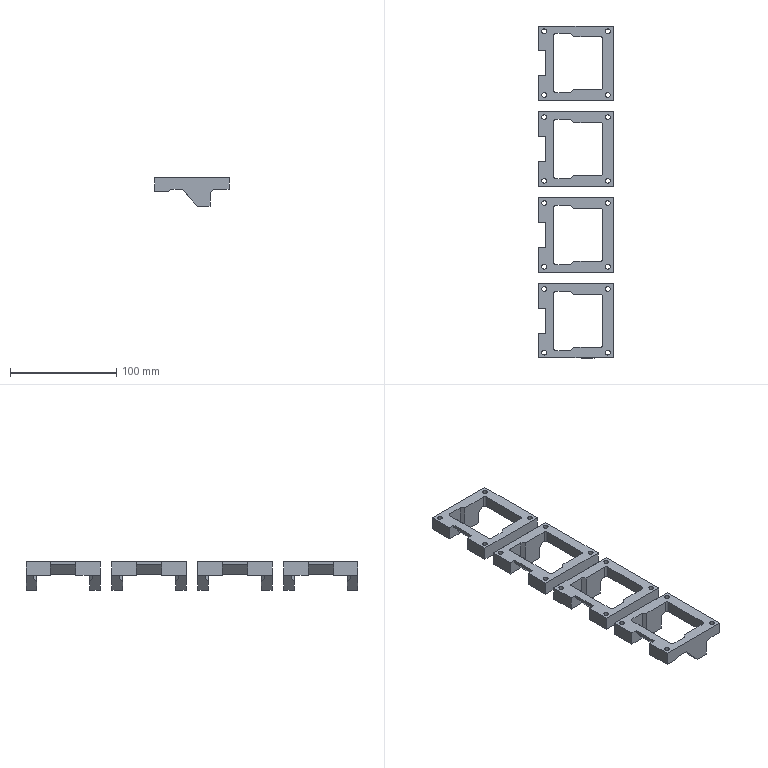NC program | NX | posted with a generic post | part box 70 x 313 x 26.9 mm
Lines 23251 to 24227 of 34421:
(CAVITY_MILL_COPY , TOOL : D4)
N46476 T04 M6
N46478 G54
N46480 G17 G0 G90 X145.982 Y5.441 S9500 M3
N46482 G43 Z30. H4
N46484 Z-11.1
N46486 G94 G1 Z-11.6 F1000.
N46488 X146.316 Y5.352
N46490 G3 X147.282 Y5.611 R1.
N46492 G1 X147.69 Y6.018 F1500.
N46494 G2 X147.987 Y6.482 R1.989
N46496 G3 X148.172 Y7.464 R1.
N46498 G1 X148.12 Y7.612
N46500 Z-11.1
N46502 G0 X145.602 Y5.062 Z-11.5
N46504 G1 Z-12. F1000.
N46506 X145.937 Y4.972
N46508 G3 X146.903 Y5.231 R1.
N46510 G1 X147.529 Y5.857 F1500.
N46512 G2 X147.789 Y6.558 R2.001
N46514 G3 X147.81 Y7.558 R1.
N46516 G1 X147.734 Y7.695
N46518 Z-11.5
N46520 G0 X145.414 Y4.874 Z-11.9
N46522 G1 Z-12.4 F1000.
N46524 X145.749 Y4.784
N46526 G3 X146.714 Y5.043 R1.
N46528 G1 X147.506 Y5.835 F1500.
N46530 G2 X147.681 Y6.704 R1.968
N46532 G3 X147.583 Y7.699 R1.
N46534 G1 X147.493 Y7.825
N46536 Z-11.9
N46538 G0 X145.304 Y4.764 Z-12.3
N46540 G1 Z-12.8 F1000.
N46542 X145.638 Y4.674
N46544 G3 X146.604 Y4.933 R1.
N46546 G1 X147.506 Y5.835 F1500.
N46548 X147.5 Y5.88
N46550 Y6.218
N46552 G2 X147.606 Y6.861 R2.
N46554 G3 X147.411 Y7.842 R1.
N46556 G1 X147.308 Y7.96
N46558 Z-12.3
N46560 G0 X145.243 Y4.703 Z-12.7
N46562 G1 Z-13.2 F1000.
N46564 X145.578 Y4.614
N46566 G3 X146.544 Y4.872 R1.
N46568 G1 X147.506 Y5.835 F1500.
N46570 X147.5 Y5.88
N46572 Y6.566
N46574 G2 X147.559 Y7.046 R2.
N46576 G3 X147.281 Y8.007 R1.
N46578 G1 X147.168 Y8.116
N46580 Z-12.7
N46582 G0 X145.219 Y4.679 Z-13.1
N46584 G1 Z-13.6 F1000.
N46586 X145.553 Y4.589
N46588 G3 X146.519 Y4.848 R1.
N46590 G1 X147.503 Y5.831 F1500.
N46592 X147.5 Y5.88
N46594 Y6.914
N46596 G2 X147.518 Y7.18 R2.
N46598 G3 X147.137 Y8.105 R1.
N46600 G1 X147.013 Y8.2
N46602 Z-13.1
N46604 G0 X145.215 Y4.675 Z-13.5
N46606 G1 Z-14. F1000.
N46608 X145.55 Y4.585
N46610 G3 X146.516 Y4.844 R1.
N46612 G1 X147.503 Y5.831 F1500.
N46614 X147.5 Y5.88
N46616 Y7.206
N46618 G3 X147. Y8.072 R1.
N46620 G1 X146.849 Y8.159
N46622 Z-13.5
N46624 G0 X145.215 Y4.675 Z-13.9
N46626 G1 Z-14.4 F1000.
N46628 X145.55 Y4.585
N46630 G3 X146.516 Y4.844 R1.
N46632 G1 X147.502 Y5.831 F1500.
N46634 X147.5 Y5.88
N46636 Y7.206
N46638 G3 X147. Y8.072 R1.
N46640 G1 X146.765 Y8.208
N46642 Z-13.9
N46644 G0 X145.215 Y4.675 Z-14.3
N46646 G1 Z-14.8 F1000.
N46648 X145.55 Y4.585
N46650 G3 X146.516 Y4.844 R1.
N46652 G1 X147.502 Y5.831 F1500.
N46654 X147.5 Y5.88
N46656 Y7.206
N46658 G3 X147. Y8.072 R1.
N46660 G1 X146.714 Y8.238
N46662 Z-14.3
N46664 G0 X145.215 Y4.675 Z-14.7
N46666 G1 Z-15.2 F1000.
N46668 X145.55 Y4.585
N46670 G3 X146.515 Y4.844 R1.
N46672 G1 X147.502 Y5.831 F1500.
N46674 X147.5 Y5.88
N46676 Y7.207
N46678 G3 X147. Y8.073 R1.
N46680 G1 X146.7 Y8.246
N46682 Z-14.7
N46684 G0 X145.215 Y4.675 Z-15.1
N46686 G1 Z-15.6 F1000.
N46688 X145.549 Y4.585
N46690 G3 X146.515 Y4.844 R1.
N46692 G1 X147.502 Y5.831 F1500.
N46694 X147.5 Y5.88
N46696 Y7.207
N46698 G3 X147. Y8.073 R1.
N46700 G1 X146.7 Y8.247
N46702 Z-15.1
N46704 G0 X145.215 Y4.675 Z-15.5
N46706 G1 Z-16. F1000.
N46708 X145.549 Y4.585
N46710 G3 X146.515 Y4.844 R1.
N46712 G1 X147.502 Y5.831 F1500.
N46714 X147.5 Y5.88
N46716 Y7.208
N46718 G3 X147. Y8.074 R1.
N46720 G1 X146.7 Y8.247
N46722 Z-15.5
N46724 G0 X145.215 Y4.675 Z-15.889
N46726 G1 Z-16.389 F1000.
N46728 X145.549 Y4.585
N46730 G3 X146.515 Y4.844 R1.
N46732 G1 X147.502 Y5.831 F1500.
N46734 X147.5 Y5.88
N46736 Y7.208
N46738 G3 X147. Y8.074 R1.
N46740 G1 X146.7 Y8.247
N46742 Z-15.889
N46744 G0 X145.215 Y4.674 Z-16.279
N46746 G1 Z-16.779 F1000.
N46748 X145.549 Y4.585
N46750 G3 X146.515 Y4.844 R1.
N46752 G1 X147.502 Y5.831 F1500.
N46754 X147.5 Y5.88
N46756 Y7.209
N46758 G3 X147. Y8.075 R1.
N46760 G1 X146.7 Y8.248
N46762 Z-16.279
N46764 G0 X145.215 Y4.674 Z-16.668
N46766 G1 Z-17.168 F1000.
N46768 X145.549 Y4.585
N46770 G3 X146.515 Y4.844 R1.
N46772 G1 X147.502 Y5.831 F1500.
N46774 X147.5 Y5.88
N46776 Y7.209
N46778 G3 X147. Y8.075 R1.
N46780 G1 X146.7 Y8.248
N46782 Z-16.668
N46784 G0 X145.215 Y4.674 Z-17.057
N46786 G1 Z-17.557 F1000.
N46788 X145.549 Y4.585
N46790 G3 X146.515 Y4.843 R1.
N46792 G1 X147.502 Y5.83 F1500.
N46794 X147.5 Y5.88
N46796 Y7.21
N46798 G3 X147. Y8.076 R1.
N46800 G1 X146.7 Y8.249
N46802 Z-17.057
N46804 G0 X145.214 Y4.674 Z-17.446
N46806 G1 Z-17.946 F1000.
N46808 X145.549 Y4.585
N46810 G3 X146.515 Y4.843 R1.
N46812 G1 X147.502 Y5.83 F1500.
N46814 X147.5 Y5.88
N46816 Y7.21
N46818 G3 X147. Y8.076 R1.
N46820 G1 X146.7 Y8.249
N46822 Z-17.446
N46824 G0 X145.214 Y4.674 Z-17.836
N46826 G1 Z-18.336 F1000.
N46828 X145.549 Y4.585
N46830 G3 X146.515 Y4.843 R1.
N46832 G1 X147.502 Y5.83 F1500.
N46834 X147.5 Y5.88
N46836 Y7.21
N46838 G3 X147. Y8.076 R1.
N46840 G1 X146.7 Y8.25
N46842 Z-17.836
N46844 G0 X145.214 Y4.674 Z-18.225
N46846 G1 Z-18.725 F1000.
N46848 X145.549 Y4.584
N46850 G3 X146.515 Y4.843 R1.
N46852 G1 X147.502 Y5.83 F1500.
N46854 X147.5 Y5.88
N46856 Y7.211
N46858 G3 X147. Y8.077 R1.
N46860 G1 X146.7 Y8.25
N46862 Z-18.225
N46864 G0 X145.214 Y4.674 Z-18.614
N46866 G1 Z-19.114 F1000.
N46868 X145.549 Y4.584
N46870 G3 X146.515 Y4.843 R1.
N46872 G1 X147.502 Y5.83 F1500.
N46874 X147.5 Y5.88
N46876 Y7.211
N46878 G3 X147. Y8.077 R1.
N46880 G1 X146.7 Y8.251
N46882 Z-18.614
N46884 G0 X145.214 Y4.674 Z-19.004
N46886 G1 Z-19.504 F1000.
N46888 X145.549 Y4.584
N46890 G3 X146.515 Y4.843 R1.
N46892 G1 X147.502 Y5.83 F1500.
N46894 X147.5 Y5.88
N46896 Y7.212
N46898 G3 X147. Y8.078 R1.
N46900 G1 X146.7 Y8.251
N46902 Z-19.004
N46904 G0 X145.214 Y4.674 Z-19.393
N46906 G1 Z-19.893 F1000.
N46908 X145.549 Y4.584
N46910 G3 X146.515 Y4.843 R1.
N46912 G1 X147.502 Y5.83 F1500.
N46914 X147.5 Y5.88
N46916 Y7.212
N46918 G3 X147. Y8.078 R1.
N46920 G1 X146.7 Y8.251
N46922 Z-19.393
N46924 G0 X145.214 Y4.674 Z-19.782
N46926 G1 Z-20.282 F1000.
N46928 X145.549 Y4.584
N46930 G3 X146.515 Y4.843 R1.
N46932 G1 X147.502 Y5.83 F1500.
N46934 X147.5 Y5.88
N46936 Y7.213
N46938 G3 X147. Y8.079 R1.
N46940 G1 X146.7 Y8.252
N46942 Z-19.782
N46944 G0 X145.214 Y4.674 Z-20.171
N46946 G1 Z-20.671 F1000.
N46948 X145.549 Y4.584
N46950 G3 X146.515 Y4.843 R1.
N46952 G1 X147.502 Y5.83 F1500.
N46954 X147.5 Y5.88
N46956 Y7.213
N46958 G3 X147. Y8.079 R1.
N46960 G1 X146.7 Y8.252
N46962 Z-20.171
N46964 G0 X145.214 Y4.674 Z-20.561
N46966 G1 Z-21.061 F1000.
N46968 X145.549 Y4.584
N46970 G3 X146.515 Y4.843 R1.
N46972 G1 X147.502 Y5.83 F1500.
N46974 X147.5 Y5.88
N46976 Y7.214
N46978 G3 X147. Y8.08 R1.
N46980 G1 X146.7 Y8.253
N46982 Z-20.561
N46984 G0 X145.214 Y4.674 Z-20.95
N46986 G1 Z-21.45 F1000.
N46988 X145.549 Y4.584
N46990 G3 X146.514 Y4.843 R1.
N46992 G1 X147.501 Y5.83 F1500.
N46994 X147.5 Y5.88
N46996 Y7.214
N46998 G3 X147. Y8.08 R1.
N47000 G1 X146.7 Y8.253
N47002 Z-20.95
N47004 G0 X145.214 Y4.674 Z-21.339
N47006 G1 Z-21.839 F1000.
N47008 X145.548 Y4.584
N47010 G3 X146.514 Y4.843 R1.
N47012 G1 X147.501 Y5.83 F1500.
N47014 X147.5 Y5.88
N47016 Y7.214
N47018 G3 X147. Y8.081 R1.
N47020 G1 X146.7 Y8.254
N47022 Z-21.339
N47024 G0 X145.214 Y4.674 Z-21.729
N47026 G1 Z-22.229 F1000.
N47028 X145.548 Y4.584
N47030 G3 X146.514 Y4.843 R1.
N47032 G1 X147.501 Y5.83 F1500.
N47034 X147.5 Y5.88
N47036 Y7.215
N47038 G3 X147. Y8.081 R1.
N47040 G1 X146.7 Y8.254
N47042 Z-21.729
N47044 G0 X145.214 Y4.674 Z-22.118
N47046 G1 Z-22.618 F1000.
N47048 X145.548 Y4.584
N47050 G3 X146.514 Y4.843 R1.
N47052 G1 X147.501 Y5.83 F1500.
N47054 X147.5 Y5.88
N47056 Y7.215
N47058 G3 X147. Y8.081 R1.
N47060 G1 X146.7 Y8.255
N47062 Z-22.118
N47064 G0 X145.214 Y4.673 Z-22.507
N47066 G1 Z-23.007 F1000.
N47068 X145.548 Y4.584
N47070 G3 X146.514 Y4.843 R1.
N47072 G1 X147.501 Y5.83 F1500.
N47074 X147.5 Y5.88
N47076 Y7.216
N47078 G3 X147. Y8.082 R1.
N47080 G1 X146.7 Y8.255
N47082 Z-22.507
N47084 G0 X145.214 Y4.673 Z-22.896
N47086 G1 Z-23.396 F1000.
N47088 X145.548 Y4.584
N47090 G3 X146.514 Y4.843 R1.
N47092 G1 X147.501 Y5.83 F1500.
N47094 X147.5 Y5.88
N47096 Y7.216
N47098 G3 X147. Y8.082 R1.
N47100 G1 X146.7 Y8.256
N47102 Z-22.896
N47104 G0 X145.214 Y4.673 Z-23.286
N47106 G1 Z-23.786 F1000.
N47108 X145.548 Y4.584
N47110 G3 X146.514 Y4.843 R1.
N47112 G1 X147.501 Y5.83 F1500.
N47114 X147.5 Y5.88
N47116 Y7.217
N47118 G3 X147. Y8.083 R1.
N47120 G1 X146.7 Y8.256
N47122 Z-23.286
N47124 G0 X145.214 Y4.673 Z-23.675
N47126 G1 Z-24.175 F1000.
N47128 X145.548 Y4.584
N47130 G3 X146.514 Y4.842 R1.
N47132 G1 X147.501 Y5.83 F1500.
N47134 X147.5 Y5.88
N47136 Y7.217
N47138 G3 X147. Y8.083 R1.
N47140 G1 X146.7 Y8.256
N47142 Z-23.675
N47144 G0 X145.213 Y4.673 Z-24.064
N47146 G1 Z-24.564 F1000.
N47148 X145.548 Y4.584
N47150 G3 X146.514 Y4.842 R1.
N47152 G1 X147.501 Y5.829 F1500.
N47154 X147.5 Y5.88
N47156 Y7.218
N47158 G3 X147. Y8.084 R1.
N47160 G1 X146.7 Y8.257
N47162 Z-24.064
N47164 G0 X145.213 Y4.673 Z-24.454
N47166 G1 Z-24.954 F1000.
N47168 X145.548 Y4.584
N47170 G3 X146.514 Y4.842 R1.
N47172 G1 X147.501 Y5.829 F1500.
N47174 X147.5 Y5.88
N47176 Y7.218
N47178 G3 X147. Y8.084 R1.
N47180 G1 X146.7 Y8.257
N47182 Z-24.454
N47184 G0 X145.213 Y4.673 Z-24.843
N47186 G1 Z-25.343 F1000.
N47188 X145.548 Y4.583
N47190 G3 X146.514 Y4.842 R1.
N47192 G1 X147.501 Y5.829 F1500.
N47194 X147.5 Y5.88
N47196 Y7.219
N47198 G3 X147. Y8.085 R1.
N47200 G1 X146.7 Y8.258
N47202 Z-24.843
N47204 G0 X145.213 Y4.673 Z-25.232
N47206 G1 Z-25.732 F1000.
N47208 X145.548 Y4.583
N47210 G3 X146.514 Y4.842 R1.
N47212 G1 X147.501 Y5.829 F1500.
N47214 X147.5 Y5.88
N47216 Y7.219
N47218 G3 X147. Y8.085 R1.
N47220 G1 X146.7 Y8.258
N47222 Z-25.232
N47224 G0 X145.213 Y4.673 Z-25.621
N47226 G1 Z-26.121 F1000.
N47228 X145.548 Y4.583
N47230 G3 X146.514 Y4.842 R1.
N47232 G1 X147.501 Y5.829 F1500.
N47234 X147.5 Y5.88
N47236 Y7.219
N47238 G3 X147. Y8.085 R1.
N47240 G1 X146.7 Y8.259
N47242 Z-25.621
N47244 G0 X145.213 Y4.673 Z-26.011
N47246 G1 Z-26.511 F1000.
N47248 X145.548 Y4.583
N47250 G3 X146.514 Y4.842 R1.
N47252 G1 X147.501 Y5.829 F1500.
N47254 X147.5 Y5.88
N47256 Y7.22
N47258 G3 X147. Y8.086 R1.
N47260 G1 X146.7 Y8.259
N47262 Z-26.011
N47264 G0 X145.213 Y4.673 Z-26.4
N47266 G1 Z-26.9 F1000.
N47268 X145.548 Y4.583
N47270 G3 X146.514 Y4.842 R1.
N47272 G1 X147.501 Y5.829 F1500.
N47274 X147.5 Y5.88
N47276 Y7.22
N47278 G3 X147. Y8.086 R1.
N47280 G1 X146.7 Y8.26
N47282 Z-26.4
N47284 G0 Z30.
N47286 X148.906 Y17.66
N47288 Z-15.1
N47290 G1 Z-15.6 F1000.
N47292 X148.875 Y17.817
N47294 G3 X148.217 Y18.571 R1.
N47296 G2 X147.493 Y19. R2.058 F1500.
N47298 G1 X146.455
N47300 G3 X145.589 Y18.5 R1.
N47302 G1 X145.415 Y18.2
N47304 Z-15.1
N47306 G0 X148.788 Y17.239 Z-15.5
N47308 G1 Z-16. F1000.
N47310 X148.784 Y17.398
N47312 G3 X148.265 Y18.253 R1.
N47314 G2 X147.493 Y19. R2.029 F1500.
N47316 G1 X146.081
N47318 G3 X145.215 Y18.5 R1.
N47320 G1 X145.041 Y18.2
N47322 Z-15.5
N47324 G0 X146.7 Y14.808 Z-15.889
N47326 G1 Z-16.389 F1000.
N47328 X147. Y14.981
N47330 G3 X147.5 Y15.847 R1.
N47332 G1 Y18.988 F1500.
N47334 X147.493 Y19.
N47336 X144.347
N47338 G3 X143.481 Y18.5 R1.
N47340 G1 X143.308 Y18.2
N47342 Z-15.889
N47344 G0 X146.7 Y14.808 Z-16.279
N47346 G1 Z-16.779 F1000.
N47348 X147. Y14.981
N47350 G3 X147.5 Y15.847 R1.
N47352 G1 Y18.988 F1500.
N47354 X147.493 Y19.
N47356 X144.347
N47358 G3 X143.481 Y18.5 R1.
N47360 G1 X143.308 Y18.2
N47362 Z-16.279
N47364 G0 X146.7 Y14.808 Z-16.668
N47366 G1 Z-17.168 F1000.
N47368 X147. Y14.981
N47370 G3 X147.5 Y15.847 R1.
N47372 G1 Y18.988 F1500.
N47374 X147.493 Y19.
N47376 X144.347
N47378 G3 X143.481 Y18.5 R1.
N47380 G1 X143.308 Y18.2
N47382 Z-16.668
N47384 G0 X146.7 Y14.808 Z-17.057
N47386 G1 Z-17.557 F1000.
N47388 X147. Y14.981
N47390 G3 X147.5 Y15.847 R1.
N47392 G1 Y18.988 F1500.
N47394 X147.493 Y19.
N47396 X144.347
N47398 G3 X143.481 Y18.5 R1.
N47400 G1 X143.308 Y18.2
N47402 Z-17.057
N47404 G0 X146.7 Y14.808 Z-17.446
N47406 G1 Z-17.946 F1000.
N47408 X147. Y14.981
N47410 G3 X147.5 Y15.847 R1.
N47412 G1 Y18.988 F1500.
N47414 X147.493 Y19.
N47416 X144.347
N47418 G3 X143.481 Y18.5 R1.
N47420 G1 X143.308 Y18.2
N47422 Z-17.446
N47424 G0 X146.7 Y14.808 Z-17.836
N47426 G1 Z-18.336 F1000.
N47428 X147. Y14.981
N47430 G3 X147.5 Y15.847 R1.
N47432 G1 Y18.988 F1500.
N47434 X147.493 Y19.
N47436 X144.347
N47438 G3 X143.481 Y18.5 R1.
N47440 G1 X143.308 Y18.2
N47442 Z-17.836
N47444 G0 X146.7 Y14.808 Z-18.225
N47446 G1 Z-18.725 F1000.
N47448 X147. Y14.981
N47450 G3 X147.5 Y15.847 R1.
N47452 G1 Y18.988 F1500.
N47454 X147.492 Y19.
N47456 X144.347
N47458 G3 X143.481 Y18.5 R1.
N47460 G1 X143.308 Y18.2
N47462 Z-18.225
N47464 G0 X146.7 Y14.808 Z-18.614
N47466 G1 Z-19.114 F1000.
N47468 X147. Y14.981
N47470 G3 X147.5 Y15.847 R1.
N47472 G1 Y18.988 F1500.
N47474 X147.492 Y19.
N47476 X144.347
N47478 G3 X143.481 Y18.5 R1.
N47480 G1 X143.308 Y18.2
N47482 Z-18.614
N47484 G0 X146.7 Y14.808 Z-19.004
N47486 G1 Z-19.504 F1000.
N47488 X147. Y14.981
N47490 G3 X147.5 Y15.847 R1.
N47492 G1 Y18.988 F1500.
N47494 X147.492 Y19.
N47496 X144.347
N47498 G3 X143.481 Y18.5 R1.
N47500 G1 X143.308 Y18.2
N47502 Z-19.004
N47504 G0 X146.7 Y14.808 Z-19.393
N47506 G1 Z-19.893 F1000.
N47508 X147. Y14.981
N47510 G3 X147.5 Y15.847 R1.
N47512 G1 Y18.988 F1500.
N47514 X147.492 Y19.
N47516 X144.347
N47518 G3 X143.481 Y18.5 R1.
N47520 G1 X143.308 Y18.2
N47522 Z-19.393
N47524 G0 X146.7 Y14.808 Z-19.782
N47526 G1 Z-20.282 F1000.
N47528 X147. Y14.981
N47530 G3 X147.5 Y15.847 R1.
N47532 G1 Y18.988 F1500.
N47534 X147.492 Y19.
N47536 X144.347
N47538 G3 X143.481 Y18.5 R1.
N47540 G1 X143.308 Y18.2
N47542 Z-19.782
N47544 G0 X146.7 Y14.808 Z-20.171
N47546 G1 Z-20.671 F1000.
N47548 X147. Y14.981
N47550 G3 X147.5 Y15.847 R1.
N47552 G1 Y18.988 F1500.
N47554 X147.492 Y19.
N47556 X144.347
N47558 G3 X143.481 Y18.5 R1.
N47560 G1 X143.308 Y18.2
N47562 Z-20.171
N47564 G0 X146.7 Y14.808 Z-20.561
N47566 G1 Z-21.061 F1000.
N47568 X147. Y14.981
N47570 G3 X147.5 Y15.847 R1.
N47572 G1 Y18.988 F1500.
N47574 X147.492 Y19.
N47576 X144.347
N47578 G3 X143.481 Y18.5 R1.
N47580 G1 X143.308 Y18.2
N47582 Z-20.561
N47584 G0 X146.7 Y14.808 Z-20.95
N47586 G1 Z-21.45 F1000.
N47588 X147. Y14.981
N47590 G3 X147.5 Y15.847 R1.
N47592 G1 Y18.988 F1500.
N47594 X147.492 Y19.
N47596 X144.347
N47598 G3 X143.481 Y18.5 R1.
N47600 G1 X143.308 Y18.2
N47602 Z-20.95
N47604 G0 X146.7 Y14.808 Z-21.339
N47606 G1 Z-21.839 F1000.
N47608 X147. Y14.981
N47610 G3 X147.5 Y15.847 R1.
N47612 G1 Y18.988 F1500.
N47614 X147.492 Y19.
N47616 X144.347
N47618 G3 X143.481 Y18.5 R1.
N47620 G1 X143.308 Y18.2
N47622 Z-21.339
N47624 G0 X146.7 Y14.808 Z-21.729
N47626 G1 Z-22.229 F1000.
N47628 X147. Y14.981
N47630 G3 X147.5 Y15.847 R1.
N47632 G1 Y18.988 F1500.
N47634 X147.492 Y19.
N47636 X144.347
N47638 G3 X143.481 Y18.5 R1.
N47640 G1 X143.308 Y18.2
N47642 Z-21.729
N47644 G0 X146.7 Y14.808 Z-22.118
N47646 G1 Z-22.618 F1000.
N47648 X147. Y14.981
N47650 G3 X147.5 Y15.847 R1.
N47652 G1 Y18.988 F1500.
N47654 X147.492 Y19.
N47656 X144.347
N47658 G3 X143.481 Y18.5 R1.
N47660 G1 X143.308 Y18.2
N47662 Z-22.118
N47664 G0 X146.7 Y14.808 Z-22.507
N47666 G1 Z-23.007 F1000.
N47668 X147. Y14.981
N47670 G3 X147.5 Y15.847 R1.
N47672 G1 Y18.988 F1500.
N47674 X147.492 Y19.
N47676 X144.347
N47678 G3 X143.481 Y18.5 R1.
N47680 G1 X143.308 Y18.2
N47682 Z-22.507
N47684 G0 X146.7 Y14.808 Z-22.896
N47686 G1 Z-23.396 F1000.
N47688 X147. Y14.981
N47690 G3 X147.5 Y15.847 R1.
N47692 G1 Y18.988 F1500.
N47694 X147.492 Y19.
N47696 X144.347
N47698 G3 X143.481 Y18.5 R1.
N47700 G1 X143.308 Y18.2
N47702 Z-22.896
N47704 G0 X146.7 Y14.808 Z-23.286
N47706 G1 Z-23.786 F1000.
N47708 X147. Y14.981
N47710 G3 X147.5 Y15.847 R1.
N47712 G1 Y18.988 F1500.
N47714 X147.492 Y19.
N47716 X144.347
N47718 G3 X143.481 Y18.5 R1.
N47720 G1 X143.308 Y18.2
N47722 Z-23.286
N47724 G0 X146.7 Y14.808 Z-23.675
N47726 G1 Z-24.175 F1000.
N47728 X147. Y14.981
N47730 G3 X147.5 Y15.847 R1.
N47732 G1 Y18.988 F1500.
N47734 X147.491 Y19.
N47736 X144.347
N47738 G3 X143.481 Y18.5 R1.
N47740 G1 X143.308 Y18.2
N47742 Z-23.675
N47744 G0 X146.7 Y14.808 Z-24.064
N47746 G1 Z-24.564 F1000.
N47748 X147. Y14.981
N47750 G3 X147.5 Y15.847 R1.
N47752 G1 Y18.988 F1500.
N47754 X147.491 Y19.
N47756 X144.347
N47758 G3 X143.481 Y18.5 R1.
N47760 G1 X143.308 Y18.2
N47762 Z-24.064
N47764 G0 X146.7 Y14.808 Z-24.454
N47766 G1 Z-24.954 F1000.
N47768 X147. Y14.981
N47770 G3 X147.5 Y15.847 R1.
N47772 G1 Y18.988 F1500.
N47774 X147.491 Y19.
N47776 X144.347
N47778 G3 X143.481 Y18.5 R1.
N47780 G1 X143.308 Y18.2
N47782 Z-24.454
N47784 G0 X146.7 Y14.808 Z-24.843
N47786 G1 Z-25.343 F1000.
N47788 X147. Y14.981
N47790 G3 X147.5 Y15.847 R1.
N47792 G1 Y18.988 F1500.
N47794 X147.491 Y19.
N47796 X144.347
N47798 G3 X143.481 Y18.5 R1.
N47800 G1 X143.308 Y18.2
N47802 Z-24.843
N47804 G0 X146.7 Y14.808 Z-25.232
N47806 G1 Z-25.732 F1000.
N47808 X147. Y14.981
N47810 G3 X147.5 Y15.847 R1.
N47812 G1 Y18.988 F1500.
N47814 X147.491 Y19.
N47816 X144.347
N47818 G3 X143.481 Y18.5 R1.
N47820 G1 X143.308 Y18.2
N47822 Z-25.232
N47824 G0 X146.7 Y14.808 Z-25.621
N47826 G1 Z-26.121 F1000.
N47828 X147. Y14.981
N47830 G3 X147.5 Y15.847 R1.
N47832 G1 Y18.988 F1500.
N47834 X147.491 Y19.
N47836 X144.347
N47838 G3 X143.481 Y18.5 R1.
N47840 G1 X143.308 Y18.2
N47842 Z-25.621
N47844 G0 X146.7 Y14.808 Z-26.011
N47846 G1 Z-26.511 F1000.
N47848 X147. Y14.981
N47850 G3 X147.5 Y15.847 R1.
N47852 G1 Y18.988 F1500.
N47854 X147.491 Y19.
N47856 X144.347
N47858 G3 X143.481 Y18.5 R1.
N47860 G1 X143.308 Y18.2
N47862 Z-26.011
N47864 G0 X146.7 Y14.808 Z-26.4
N47866 G1 Z-26.9 F1000.
N47868 X147. Y14.981
N47870 G3 X147.5 Y15.847 R1.
N47872 G1 Y18.988 F1500.
N47874 X147.491 Y19.
N47876 X144.347
N47878 G3 X143.481 Y18.5 R1.
N47880 G1 X143.308 Y18.2
N47882 Z-26.4
N47884 G0 Z30.
N47886 X127.308 Y24.355
N47888 Z-14.7
N47890 G1 Z-15.2 F1000.
N47892 X127.481 Y24.055
N47894 G3 X128.347 Y23.555 R1.
N47896 G1 X131.5 F1500.
N47898 Y26.708
N47900 G3 X131. Y27.574 R1.
N47902 G1 X130.7 Y27.747
N47904 Z-14.7
N47906 G0 X127.308 Y24.702 Z-15.1
N47908 G1 Z-15.6 F1000.
N47910 X127.481 Y24.402
N47912 G3 X128.347 Y23.902 R1.
N47914 G1 X131.5 F1500.
N47916 Y27.055
N47918 G3 X131. Y27.921 R1.
N47920 G1 X130.7 Y28.095
N47922 Z-15.1
N47924 G0 X127.308 Y25.048 Z-15.5
N47926 G1 Z-16. F1000.
N47928 X127.481 Y24.748
N47930 G3 X128.347 Y24.248 R1.
N47932 G1 X131.5 F1500.
N47934 Y27.401
N47936 G3 X131. Y28.267 R1.
N47938 G1 X130.7 Y28.44
N47940 Z-15.5
N47942 G0 X127.308 Y25.389 Z-15.889
N47944 G1 Z-16.389 F1000.
N47946 X127.481 Y25.089
N47948 G3 X128.347 Y24.589 R1.
N47950 G1 X131.5 F1500.
N47952 Y27.742
N47954 G3 X131. Y28.608 R1.
N47956 G1 X130.7 Y28.781
N47958 Z-15.889
N47960 G0 X127.308 Y25.727 Z-16.279
N47962 G1 Z-16.779 F1000.
N47964 X127.481 Y25.427
N47966 G3 X128.347 Y24.927 R1.
N47968 G1 X131.5 F1500.
N47970 Y28.08
N47972 G3 X131. Y28.946 R1.
N47974 G1 X130.7 Y29.119
N47976 Z-16.279
N47978 G0 X127.308 Y26.065 Z-16.668
N47980 G1 Z-17.168 F1000.
N47982 X127.481 Y25.765
N47984 G3 X128.347 Y25.265 R1.
N47986 G1 X131.5 F1500.
N47988 Y28.418
N47990 G3 X131. Y29.284 R1.
N47992 G1 X130.7 Y29.458
N47994 Z-16.668
N47996 G0 X127.308 Y26.404 Z-17.057
N47998 G1 Z-17.557 F1000.
N48000 X127.481 Y26.104
N48002 G3 X128.347 Y25.604 R1.
N48004 G1 X131.5 F1500.
N48006 Y28.757
N48008 G3 X131. Y29.623 R1.
N48010 G1 X130.7 Y29.796
N48012 Z-17.057
N48014 G0 X127.308 Y26.742 Z-17.446
N48016 G1 Z-17.946 F1000.
N48018 X127.481 Y26.442
N48020 G3 X128.347 Y25.942 R1.
N48022 G1 X131.5 F1500.
N48024 Y29.095
N48026 G3 X131. Y29.961 R1.
N48028 G1 X130.7 Y30.134
N48030 Z-17.446
N48032 G0 X127.308 Y27.081 Z-17.836
N48034 G1 Z-18.336 F1000.
N48036 X127.481 Y26.781
N48038 G3 X128.347 Y26.281 R1.
N48040 G1 X131.5 F1500.
N48042 Y29.434
N48044 G3 X131. Y30.3 R1.
N48046 G1 X130.7 Y30.473
N48048 Z-17.836
N48050 G0 X127.308 Y27.419 Z-18.225
N48052 G1 Z-18.725 F1000.
N48054 X127.481 Y27.119
N48056 G3 X128.347 Y26.619 R1.
N48058 G1 X131.5 F1500.
N48060 Y29.772
N48062 G3 X131. Y30.638 R1.
N48064 G1 X130.7 Y30.811
N48066 Z-18.225
N48068 G0 X127.308 Y27.757 Z-18.614
N48070 G1 Z-19.114 F1000.
N48072 X127.481 Y27.457
N48074 G3 X128.347 Y26.957 R1.
N48076 G1 X131.5 F1500.
N48078 Y30.11
N48080 G3 X131. Y30.976 R1.
N48082 G1 X130.7 Y31.15
N48084 Z-18.614
N48086 G0 X127.308 Y28.096 Z-19.004
N48088 G1 Z-19.504 F1000.
N48090 X127.481 Y27.796
N48092 G3 X128.347 Y27.296 R1.
N48094 G1 X131.5 F1500.
N48096 Y30.449
N48098 G3 X131. Y31.315 R1.
N48100 G1 X130.7 Y31.488
N48102 Z-19.004
N48104 G0 X127.308 Y28.434 Z-19.393
N48106 G1 Z-19.893 F1000.
N48108 X127.481 Y28.134
N48110 G3 X128.347 Y27.634 R1.
N48112 G1 X131.5 F1500.
N48114 Y30.787
N48116 G3 X131. Y31.653 R1.
N48118 G1 X130.7 Y31.826
N48120 Z-19.393
N48122 G0 X127.308 Y28.773 Z-19.782
N48124 G1 Z-20.282 F1000.
N48126 X127.481 Y28.473
N48128 G3 X128.347 Y27.973 R1.
N48130 G1 X131.5 F1500.
N48132 Y31.126
N48134 G3 X131. Y31.992 R1.
N48136 G1 X130.7 Y32.165
N48138 Z-19.782
N48140 G0 X127.308 Y29.111 Z-20.171
N48142 G1 Z-20.671 F1000.
N48144 X127.481 Y28.811
N48146 G3 X128.347 Y28.311 R1.
N48148 G1 X131.5 F1500.
N48150 Y31.464
N48152 G3 X131. Y32.33 R1.
N48154 G1 X130.7 Y32.503
N48156 Z-20.171
N48158 G0 X127.308 Y29.449 Z-20.561
N48160 G1 Z-21.061 F1000.
N48162 X127.481 Y29.149
N48164 G3 X128.347 Y28.649 R1.
N48166 G1 X131.5 F1500.
N48168 Y31.802
N48170 G3 X131. Y32.668 R1.
N48172 G1 X130.7 Y32.842
N48174 Z-20.561
N48176 G0 X127.308 Y29.788 Z-20.95
N48178 G1 Z-21.45 F1000.
N48180 X127.481 Y29.488
N48182 G3 X128.347 Y28.988 R1.
N48184 G1 X131.5 F1500.
N48186 Y32.141
N48188 G3 X131. Y33.007 R1.
N48190 G1 X130.7 Y33.18
N48192 Z-20.95
N48194 G0 X127.308 Y30.126 Z-21.339
N48196 G1 Z-21.839 F1000.
N48198 X127.481 Y29.826
N48200 G3 X128.347 Y29.326 R1.
N48202 G1 X131.5 F1500.
N48204 Y32.479
N48206 G3 X131. Y33.345 R1.
N48208 G1 X130.7 Y33.518
N48210 Z-21.339
N48212 G0 X127.308 Y30.465 Z-21.729
N48214 G1 Z-22.229 F1000.
N48216 X127.481 Y30.165
N48218 G3 X128.347 Y29.665 R1.
N48220 G1 X131.5 F1500.
N48222 Y32.818
N48224 G3 X131. Y33.684 R1.
N48226 G1 X130.7 Y33.857
N48228 Z-21.729
N48230 G0 X127.308 Y30.803 Z-22.118
N48232 G1 Z-22.618 F1000.
N48234 X127.481 Y30.503
N48236 G3 X128.347 Y30.003 R1.
N48238 G1 X131.5 F1500.
N48240 Y33.156
N48242 G3 X131. Y34.022 R1.
N48244 G1 X130.7 Y34.195
N48246 Z-22.118
N48248 G0 X127.308 Y31.141 Z-22.507
N48250 G1 Z-23.007 F1000.
N48252 X127.481 Y30.841
N48254 G3 X128.347 Y30.341 R1.
N48256 G1 X131.5 F1500.
N48258 Y33.494
N48260 G3 X131. Y34.36 R1.
N48262 G1 X130.7 Y34.534
N48264 Z-22.507
N48266 G0 X127.308 Y31.48 Z-22.896
N48268 G1 Z-23.396 F1000.
N48270 X127.481 Y31.18
N48272 G3 X128.347 Y30.68 R1.
N48274 G1 X131.5 F1500.
N48276 Y33.833
N48278 G3 X131. Y34.699 R1.
N48280 G1 X130.7 Y34.872
N48282 Z-22.896
N48284 G0 X127.308 Y31.818 Z-23.286
N48286 G1 Z-23.786 F1000.
N48288 X127.481 Y31.518
N48290 G3 X128.347 Y31.018 R1.
N48292 G1 X131.5 F1500.
N48294 Y34.171
N48296 G3 X131. Y35.037 R1.
N48298 G1 X130.708 Y35.206
N48300 Z-23.286
N48302 G0 X127.308 Y32.004 Z-23.675
N48304 G1 Z-24.175 F1000.
N48306 X127.481 Y31.704
N48308 G3 X128.347 Y31.204 R1.
N48310 G1 X131.5 F1500.
N48312 Y34.357
N48314 G3 X131. Y35.223 R1.
N48316 G1 X130.726 Y35.382
N48318 Z-23.675
N48320 G0 X127.308 Y32.004 Z-24.064
N48322 G1 Z-24.564 F1000.
N48324 X127.481 Y31.704
N48326 G3 X128.347 Y31.204 R1.
N48328 G1 X131.5 F1500.
N48330 Y34.357
N48332 G3 X131. Y35.223 R1.
N48334 G1 X130.726 Y35.382
N48336 Z-24.064
N48338 G0 X127.308 Y32.004 Z-24.454
N48340 G1 Z-24.954 F1000.
N48342 X127.481 Y31.704
N48344 G3 X128.347 Y31.204 R1.
N48346 G1 X131.5 F1500.
N48348 Y34.357
N48350 G3 X131. Y35.223 R1.
N48352 G1 X130.726 Y35.382
N48354 Z-24.454
N48356 G0 X127.308 Y32.004 Z-24.843
N48358 G1 Z-25.343 F1000.
N48360 X127.481 Y31.704
N48362 G3 X128.347 Y31.204 R1.
N48364 G1 X131.5 F1500.
N48366 Y34.357
N48368 G3 X131. Y35.223 R1.
N48370 G1 X130.726 Y35.382
N48372 Z-24.843
N48374 G0 X127.308 Y32.004 Z-25.232
N48376 G1 Z-25.732 F1000.
N48378 X127.481 Y31.704
N48380 G3 X128.347 Y31.204 R1.
N48382 G1 X131.5 F1500.
N48384 Y34.357
N48386 G3 X131. Y35.223 R1.
N48388 G1 X130.726 Y35.382
N48390 Z-25.232
N48392 G0 X127.308 Y32.004 Z-25.621
N48394 G1 Z-26.121 F1000.
N48396 X127.481 Y31.704
N48398 G3 X128.347 Y31.204 R1.
N48400 G1 X131.5 F1500.
N48402 Y34.357
N48404 G3 X131. Y35.223 R1.
N48406 G1 X130.726 Y35.382
N48408 Z-25.621
N48410 G0 X127.308 Y32.004 Z-26.011
N48412 G1 Z-26.511 F1000.
N48414 X127.481 Y31.704
N48416 G3 X128.347 Y31.204 R1.
N48418 G1 X131.5 F1500.
N48420 Y34.357
N48422 G3 X131. Y35.223 R1.